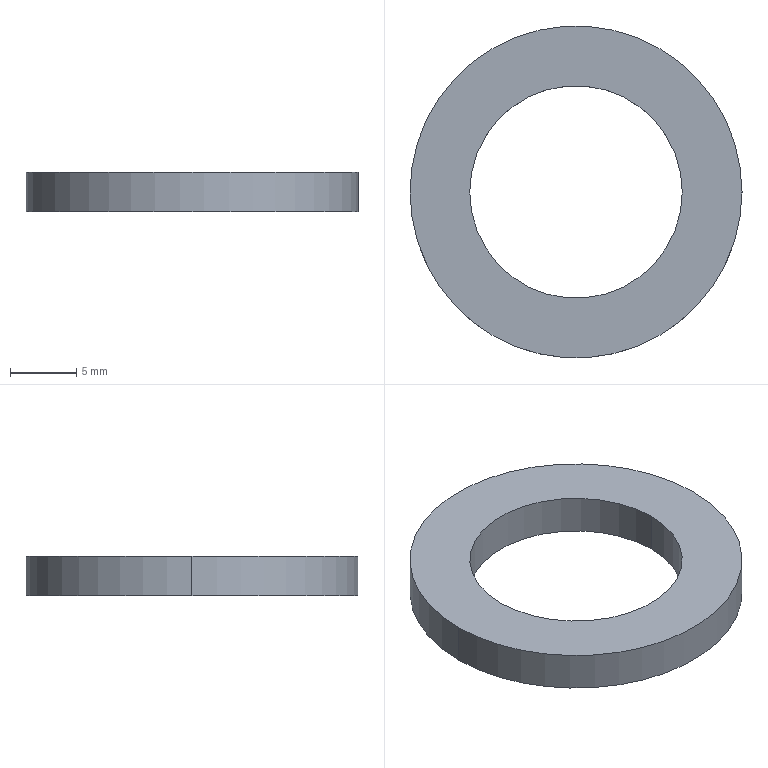Part | STEP file | Cuon T phu H01_17 | 1 solid | 6 faces | box 25 x 25 x 3 mm | volume 869.436 mm3 | cylinder 4 | plane 2 | commonest cylinder face diameters 16 x2 25 x2
STEP:
#1=CARTESIAN_POINT('',(0.,0.,0.));
#2=DIRECTION('',(0.,0.,1.));
#3=DIRECTION('',(1.,0.,0.));
#4=AXIS2_PLACEMENT_3D('',#1,#2,#3);
#5=CARTESIAN_POINT('',(-8.,0.,3.));
#6=VERTEX_POINT('',#5);
#7=CARTESIAN_POINT('',(-8.,0.,0.));
#8=VERTEX_POINT('',#7);
#9=CARTESIAN_POINT('',(-8.,0.,3.));
#10=DIRECTION('',(0.,0.,-1.));
#11=VECTOR('',#10,1.);
#12=LINE('',#9,#11);
#13=CARTESIAN_POINT('',(0.,0.,3.));
#14=DIRECTION('',(0.,0.,-1.));
#15=DIRECTION('',(-1.,0.,0.));
#16=AXIS2_PLACEMENT_3D('',#13,#14,#15);
#17=CYLINDRICAL_SURFACE('',#16,8.);
#18=CARTESIAN_POINT('',(6.283,0.));
#19=DIRECTION('',(0.,1.));
#20=VECTOR('',#19,1.);
#21=LINE('',#18,#20);
#22=(GEOMETRIC_REPRESENTATION_CONTEXT(2)PARAMETRIC_REPRESENTATION_CONTEXT()REPRESENTATION_CONTEXT('',''));
#23=DEFINITIONAL_REPRESENTATION('',(#21),#22);
#24=PCURVE('',#17,#23);
#25=CARTESIAN_POINT('',(0.,0.,3.));
#26=DIRECTION('',(0.,0.,-1.));
#27=DIRECTION('',(-1.,0.,0.));
#28=AXIS2_PLACEMENT_3D('',#25,#26,#27);
#29=CYLINDRICAL_SURFACE('',#28,8.);
#30=CARTESIAN_POINT('',(0.,0.));
#31=DIRECTION('',(0.,1.));
#32=VECTOR('',#31,1.);
#33=LINE('',#30,#32);
#34=(GEOMETRIC_REPRESENTATION_CONTEXT(2)PARAMETRIC_REPRESENTATION_CONTEXT()REPRESENTATION_CONTEXT('',''));
#35=DEFINITIONAL_REPRESENTATION('',(#33),#34);
#36=PCURVE('',#29,#35);
#37=SURFACE_CURVE('',#12,(#24,#36),.PCURVE_S1.);
#38=EDGE_CURVE('',#6,#8,#37,.T.);
#39=ORIENTED_EDGE('',*,*,#38,.T.);
#40=CARTESIAN_POINT('',(8.,0.,0.));
#41=VERTEX_POINT('',#40);
#42=CARTESIAN_POINT('',(0.,0.,0.));
#43=DIRECTION('',(0.,0.,1.));
#44=DIRECTION('',(1.,0.,0.));
#45=AXIS2_PLACEMENT_3D('',#42,#43,#44);
#46=CIRCLE('',#45,8.);
#47=CARTESIAN_POINT('',(9.425,3.));
#48=DIRECTION('',(-1.,0.));
#49=VECTOR('',#48,1.);
#50=LINE('',#47,#49);
#51=(GEOMETRIC_REPRESENTATION_CONTEXT(2)PARAMETRIC_REPRESENTATION_CONTEXT()REPRESENTATION_CONTEXT('',''));
#52=DEFINITIONAL_REPRESENTATION('',(#50),#51);
#53=PCURVE('',#17,#52);
#54=CARTESIAN_POINT('',(0.,0.,0.));
#55=DIRECTION('',(0.,0.,1.));
#56=DIRECTION('',(1.,0.,0.));
#57=AXIS2_PLACEMENT_3D('',#54,#55,#56);
#58=PLANE('',#57);
#59=CARTESIAN_POINT('',(0.,0.));
#60=DIRECTION('',(1.,0.));
#61=AXIS2_PLACEMENT_2D('',#59,#60);
#62=CIRCLE('',#61,8.);
#63=(GEOMETRIC_REPRESENTATION_CONTEXT(2)PARAMETRIC_REPRESENTATION_CONTEXT()REPRESENTATION_CONTEXT('',''));
#64=DEFINITIONAL_REPRESENTATION('',(#62),#63);
#65=PCURVE('',#58,#64);
#66=SURFACE_CURVE('',#46,(#53,#65),.PCURVE_S1.);
#67=EDGE_CURVE('',#8,#41,#66,.T.);
#68=ORIENTED_EDGE('',*,*,#67,.T.);
#69=CARTESIAN_POINT('',(8.,0.,3.));
#70=VERTEX_POINT('',#69);
#71=CARTESIAN_POINT('',(8.,0.,3.));
#72=DIRECTION('',(0.,0.,-1.));
#73=VECTOR('',#72,1.);
#74=LINE('',#71,#73);
#75=CARTESIAN_POINT('',(3.142,0.));
#76=DIRECTION('',(0.,1.));
#77=VECTOR('',#76,1.);
#78=LINE('',#75,#77);
#79=(GEOMETRIC_REPRESENTATION_CONTEXT(2)PARAMETRIC_REPRESENTATION_CONTEXT()REPRESENTATION_CONTEXT('',''));
#80=DEFINITIONAL_REPRESENTATION('',(#78),#79);
#81=PCURVE('',#17,#80);
#82=CARTESIAN_POINT('',(3.142,0.));
#83=DIRECTION('',(0.,1.));
#84=VECTOR('',#83,1.);
#85=LINE('',#82,#84);
#86=(GEOMETRIC_REPRESENTATION_CONTEXT(2)PARAMETRIC_REPRESENTATION_CONTEXT()REPRESENTATION_CONTEXT('',''));
#87=DEFINITIONAL_REPRESENTATION('',(#85),#86);
#88=PCURVE('',#29,#87);
#89=SURFACE_CURVE('',#74,(#81,#88),.PCURVE_S1.);
#90=EDGE_CURVE('',#70,#41,#89,.T.);
#91=ORIENTED_EDGE('',*,*,#90,.F.);
#92=CARTESIAN_POINT('',(0.,0.,3.));
#93=DIRECTION('',(0.,0.,1.));
#94=DIRECTION('',(1.,0.,0.));
#95=AXIS2_PLACEMENT_3D('',#92,#93,#94);
#96=CIRCLE('',#95,8.);
#97=CARTESIAN_POINT('',(9.425,0.));
#98=DIRECTION('',(-1.,0.));
#99=VECTOR('',#98,1.);
#100=LINE('',#97,#99);
#101=(GEOMETRIC_REPRESENTATION_CONTEXT(2)PARAMETRIC_REPRESENTATION_CONTEXT()REPRESENTATION_CONTEXT('',''));
#102=DEFINITIONAL_REPRESENTATION('',(#100),#101);
#103=PCURVE('',#17,#102);
#104=CARTESIAN_POINT('',(0.,0.,3.));
#105=DIRECTION('',(0.,0.,1.));
#106=DIRECTION('',(1.,0.,0.));
#107=AXIS2_PLACEMENT_3D('',#104,#105,#106);
#108=PLANE('',#107);
#109=CARTESIAN_POINT('',(0.,0.));
#110=DIRECTION('',(1.,0.));
#111=AXIS2_PLACEMENT_2D('',#109,#110);
#112=CIRCLE('',#111,8.);
#113=(GEOMETRIC_REPRESENTATION_CONTEXT(2)PARAMETRIC_REPRESENTATION_CONTEXT()REPRESENTATION_CONTEXT('',''));
#114=DEFINITIONAL_REPRESENTATION('',(#112),#113);
#115=PCURVE('',#108,#114);
#116=SURFACE_CURVE('',#96,(#103,#115),.PCURVE_S1.);
#117=EDGE_CURVE('',#6,#70,#116,.T.);
#118=ORIENTED_EDGE('',*,*,#117,.F.);
#119=EDGE_LOOP('',(#39,#68,#91,#118));
#120=FACE_BOUND('',#119,.F.);
#121=ADVANCED_FACE('',(#120),#17,.F.);
#122=CARTESIAN_POINT('',(12.5,0.,3.));
#123=VERTEX_POINT('',#122);
#124=CARTESIAN_POINT('',(-12.5,0.,3.));
#125=VERTEX_POINT('',#124);
#126=CARTESIAN_POINT('',(0.,0.,3.));
#127=DIRECTION('',(0.,0.,1.));
#128=DIRECTION('',(1.,0.,0.));
#129=AXIS2_PLACEMENT_3D('',#126,#127,#128);
#130=CIRCLE('',#129,12.5);
#131=CARTESIAN_POINT('',(0.,0.,3.));
#132=DIRECTION('',(0.,0.,-1.));
#133=DIRECTION('',(-1.,0.,0.));
#134=AXIS2_PLACEMENT_3D('',#131,#132,#133);
#135=CYLINDRICAL_SURFACE('',#134,12.5);
#136=CARTESIAN_POINT('',(3.142,0.));
#137=DIRECTION('',(-1.,0.));
#138=VECTOR('',#137,1.);
#139=LINE('',#136,#138);
#140=(GEOMETRIC_REPRESENTATION_CONTEXT(2)PARAMETRIC_REPRESENTATION_CONTEXT()REPRESENTATION_CONTEXT('',''));
#141=DEFINITIONAL_REPRESENTATION('',(#139),#140);
#142=PCURVE('',#135,#141);
#143=CARTESIAN_POINT('',(0.,0.));
#144=DIRECTION('',(1.,0.));
#145=AXIS2_PLACEMENT_2D('',#143,#144);
#146=CIRCLE('',#145,12.5);
#147=(GEOMETRIC_REPRESENTATION_CONTEXT(2)PARAMETRIC_REPRESENTATION_CONTEXT()REPRESENTATION_CONTEXT('',''));
#148=DEFINITIONAL_REPRESENTATION('',(#146),#147);
#149=PCURVE('',#108,#148);
#150=SURFACE_CURVE('',#130,(#142,#149),.PCURVE_S1.);
#151=EDGE_CURVE('',#123,#125,#150,.T.);
#152=ORIENTED_EDGE('',*,*,#151,.F.);
#153=CARTESIAN_POINT('',(12.5,0.,0.));
#154=VERTEX_POINT('',#153);
#155=CARTESIAN_POINT('',(12.5,0.,3.));
#156=DIRECTION('',(0.,0.,-1.));
#157=VECTOR('',#156,1.);
#158=LINE('',#155,#157);
#159=CARTESIAN_POINT('',(3.142,0.));
#160=DIRECTION('',(0.,1.));
#161=VECTOR('',#160,1.);
#162=LINE('',#159,#161);
#163=(GEOMETRIC_REPRESENTATION_CONTEXT(2)PARAMETRIC_REPRESENTATION_CONTEXT()REPRESENTATION_CONTEXT('',''));
#164=DEFINITIONAL_REPRESENTATION('',(#162),#163);
#165=PCURVE('',#135,#164);
#166=CARTESIAN_POINT('',(0.,0.,3.));
#167=DIRECTION('',(0.,0.,-1.));
#168=DIRECTION('',(-1.,0.,0.));
#169=AXIS2_PLACEMENT_3D('',#166,#167,#168);
#170=CYLINDRICAL_SURFACE('',#169,12.5);
#171=CARTESIAN_POINT('',(3.142,0.));
#172=DIRECTION('',(0.,1.));
#173=VECTOR('',#172,1.);
#174=LINE('',#171,#173);
#175=(GEOMETRIC_REPRESENTATION_CONTEXT(2)PARAMETRIC_REPRESENTATION_CONTEXT()REPRESENTATION_CONTEXT('',''));
#176=DEFINITIONAL_REPRESENTATION('',(#174),#175);
#177=PCURVE('',#170,#176);
#178=SURFACE_CURVE('',#158,(#165,#177),.PCURVE_S1.);
#179=EDGE_CURVE('',#123,#154,#178,.T.);
#180=ORIENTED_EDGE('',*,*,#179,.T.);
#181=CARTESIAN_POINT('',(-12.5,0.,0.));
#182=VERTEX_POINT('',#181);
#183=CARTESIAN_POINT('',(0.,0.,0.));
#184=DIRECTION('',(0.,0.,1.));
#185=DIRECTION('',(1.,0.,0.));
#186=AXIS2_PLACEMENT_3D('',#183,#184,#185);
#187=CIRCLE('',#186,12.5);
#188=CARTESIAN_POINT('',(3.142,3.));
#189=DIRECTION('',(-1.,0.));
#190=VECTOR('',#189,1.);
#191=LINE('',#188,#190);
#192=(GEOMETRIC_REPRESENTATION_CONTEXT(2)PARAMETRIC_REPRESENTATION_CONTEXT()REPRESENTATION_CONTEXT('',''));
#193=DEFINITIONAL_REPRESENTATION('',(#191),#192);
#194=PCURVE('',#135,#193);
#195=CARTESIAN_POINT('',(0.,0.));
#196=DIRECTION('',(1.,0.));
#197=AXIS2_PLACEMENT_2D('',#195,#196);
#198=CIRCLE('',#197,12.5);
#199=(GEOMETRIC_REPRESENTATION_CONTEXT(2)PARAMETRIC_REPRESENTATION_CONTEXT()REPRESENTATION_CONTEXT('',''));
#200=DEFINITIONAL_REPRESENTATION('',(#198),#199);
#201=PCURVE('',#58,#200);
#202=SURFACE_CURVE('',#187,(#194,#201),.PCURVE_S1.);
#203=EDGE_CURVE('',#154,#182,#202,.T.);
#204=ORIENTED_EDGE('',*,*,#203,.T.);
#205=CARTESIAN_POINT('',(-12.5,0.,3.));
#206=DIRECTION('',(0.,0.,-1.));
#207=VECTOR('',#206,1.);
#208=LINE('',#205,#207);
#209=CARTESIAN_POINT('',(0.,0.));
#210=DIRECTION('',(0.,1.));
#211=VECTOR('',#210,1.);
#212=LINE('',#209,#211);
#213=(GEOMETRIC_REPRESENTATION_CONTEXT(2)PARAMETRIC_REPRESENTATION_CONTEXT()REPRESENTATION_CONTEXT('',''));
#214=DEFINITIONAL_REPRESENTATION('',(#212),#213);
#215=PCURVE('',#135,#214);
#216=CARTESIAN_POINT('',(6.283,0.));
#217=DIRECTION('',(0.,1.));
#218=VECTOR('',#217,1.);
#219=LINE('',#216,#218);
#220=(GEOMETRIC_REPRESENTATION_CONTEXT(2)PARAMETRIC_REPRESENTATION_CONTEXT()REPRESENTATION_CONTEXT('',''));
#221=DEFINITIONAL_REPRESENTATION('',(#219),#220);
#222=PCURVE('',#170,#221);
#223=SURFACE_CURVE('',#208,(#215,#222),.PCURVE_S1.);
#224=EDGE_CURVE('',#125,#182,#223,.T.);
#225=ORIENTED_EDGE('',*,*,#224,.F.);
#226=EDGE_LOOP('',(#152,#180,#204,#225));
#227=FACE_BOUND('',#226,.T.);
#228=ADVANCED_FACE('',(#227),#135,.T.);
#229=CARTESIAN_POINT('',(0.,0.,3.));
#230=DIRECTION('',(0.,0.,1.));
#231=DIRECTION('',(1.,0.,0.));
#232=AXIS2_PLACEMENT_3D('',#229,#230,#231);
#233=CIRCLE('',#232,12.5);
#234=CARTESIAN_POINT('',(0.,0.));
#235=DIRECTION('',(1.,0.));
#236=AXIS2_PLACEMENT_2D('',#234,#235);
#237=CIRCLE('',#236,12.5);
#238=(GEOMETRIC_REPRESENTATION_CONTEXT(2)PARAMETRIC_REPRESENTATION_CONTEXT()REPRESENTATION_CONTEXT('',''));
#239=DEFINITIONAL_REPRESENTATION('',(#237),#238);
#240=PCURVE('',#108,#239);
#241=CARTESIAN_POINT('',(9.425,0.));
#242=DIRECTION('',(-1.,0.));
#243=VECTOR('',#242,1.);
#244=LINE('',#241,#243);
#245=(GEOMETRIC_REPRESENTATION_CONTEXT(2)PARAMETRIC_REPRESENTATION_CONTEXT()REPRESENTATION_CONTEXT('',''));
#246=DEFINITIONAL_REPRESENTATION('',(#244),#245);
#247=PCURVE('',#170,#246);
#248=SURFACE_CURVE('',#233,(#240,#247),.PCURVE_S1.);
#249=EDGE_CURVE('',#125,#123,#248,.T.);
#250=ORIENTED_EDGE('',*,*,#249,.T.);
#251=ORIENTED_EDGE('',*,*,#151,.T.);
#252=EDGE_LOOP('',(#250,#251));
#253=FACE_BOUND('',#252,.T.);
#254=ORIENTED_EDGE('',*,*,#117,.F.);
#255=CARTESIAN_POINT('',(0.,0.,3.));
#256=DIRECTION('',(0.,0.,1.));
#257=DIRECTION('',(1.,0.,0.));
#258=AXIS2_PLACEMENT_3D('',#255,#256,#257);
#259=CIRCLE('',#258,8.);
#260=CARTESIAN_POINT('',(0.,0.));
#261=DIRECTION('',(1.,0.));
#262=AXIS2_PLACEMENT_2D('',#260,#261);
#263=CIRCLE('',#262,8.);
#264=(GEOMETRIC_REPRESENTATION_CONTEXT(2)PARAMETRIC_REPRESENTATION_CONTEXT()REPRESENTATION_CONTEXT('',''));
#265=DEFINITIONAL_REPRESENTATION('',(#263),#264);
#266=PCURVE('',#108,#265);
#267=CARTESIAN_POINT('',(3.142,0.));
#268=DIRECTION('',(-1.,0.));
#269=VECTOR('',#268,1.);
#270=LINE('',#267,#269);
#271=(GEOMETRIC_REPRESENTATION_CONTEXT(2)PARAMETRIC_REPRESENTATION_CONTEXT()REPRESENTATION_CONTEXT('',''));
#272=DEFINITIONAL_REPRESENTATION('',(#270),#271);
#273=PCURVE('',#29,#272);
#274=SURFACE_CURVE('',#259,(#266,#273),.PCURVE_S1.);
#275=EDGE_CURVE('',#70,#6,#274,.T.);
#276=ORIENTED_EDGE('',*,*,#275,.F.);
#277=EDGE_LOOP('',(#254,#276));
#278=FACE_BOUND('',#277,.T.);
#279=ADVANCED_FACE('',(#253,#278),#108,.T.);
#280=CARTESIAN_POINT('',(0.,0.,0.));
#281=DIRECTION('',(0.,0.,1.));
#282=DIRECTION('',(1.,0.,0.));
#283=AXIS2_PLACEMENT_3D('',#280,#281,#282);
#284=CIRCLE('',#283,12.5);
#285=CARTESIAN_POINT('',(0.,0.));
#286=DIRECTION('',(1.,0.));
#287=AXIS2_PLACEMENT_2D('',#285,#286);
#288=CIRCLE('',#287,12.5);
#289=(GEOMETRIC_REPRESENTATION_CONTEXT(2)PARAMETRIC_REPRESENTATION_CONTEXT()REPRESENTATION_CONTEXT('',''));
#290=DEFINITIONAL_REPRESENTATION('',(#288),#289);
#291=PCURVE('',#58,#290);
#292=CARTESIAN_POINT('',(9.425,3.));
#293=DIRECTION('',(-1.,0.));
#294=VECTOR('',#293,1.);
#295=LINE('',#292,#294);
#296=(GEOMETRIC_REPRESENTATION_CONTEXT(2)PARAMETRIC_REPRESENTATION_CONTEXT()REPRESENTATION_CONTEXT('',''));
#297=DEFINITIONAL_REPRESENTATION('',(#295),#296);
#298=PCURVE('',#170,#297);
#299=SURFACE_CURVE('',#284,(#291,#298),.PCURVE_S1.);
#300=EDGE_CURVE('',#182,#154,#299,.T.);
#301=ORIENTED_EDGE('',*,*,#300,.F.);
#302=ORIENTED_EDGE('',*,*,#203,.F.);
#303=EDGE_LOOP('',(#301,#302));
#304=FACE_BOUND('',#303,.T.);
#305=ORIENTED_EDGE('',*,*,#67,.T.);
#306=CARTESIAN_POINT('',(0.,0.,0.));
#307=DIRECTION('',(0.,0.,1.));
#308=DIRECTION('',(1.,0.,0.));
#309=AXIS2_PLACEMENT_3D('',#306,#307,#308);
#310=CIRCLE('',#309,8.);
#311=CARTESIAN_POINT('',(0.,0.));
#312=DIRECTION('',(1.,0.));
#313=AXIS2_PLACEMENT_2D('',#311,#312);
#314=CIRCLE('',#313,8.);
#315=(GEOMETRIC_REPRESENTATION_CONTEXT(2)PARAMETRIC_REPRESENTATION_CONTEXT()REPRESENTATION_CONTEXT('',''));
#316=DEFINITIONAL_REPRESENTATION('',(#314),#315);
#317=PCURVE('',#58,#316);
#318=CARTESIAN_POINT('',(3.142,3.));
#319=DIRECTION('',(-1.,0.));
#320=VECTOR('',#319,1.);
#321=LINE('',#318,#320);
#322=(GEOMETRIC_REPRESENTATION_CONTEXT(2)PARAMETRIC_REPRESENTATION_CONTEXT()REPRESENTATION_CONTEXT('',''));
#323=DEFINITIONAL_REPRESENTATION('',(#321),#322);
#324=PCURVE('',#29,#323);
#325=SURFACE_CURVE('',#310,(#317,#324),.PCURVE_S1.);
#326=EDGE_CURVE('',#41,#8,#325,.T.);
#327=ORIENTED_EDGE('',*,*,#326,.T.);
#328=EDGE_LOOP('',(#305,#327));
#329=FACE_BOUND('',#328,.T.);
#330=ADVANCED_FACE('',(#304,#329),#58,.F.);
#331=ORIENTED_EDGE('',*,*,#179,.F.);
#332=ORIENTED_EDGE('',*,*,#249,.F.);
#333=ORIENTED_EDGE('',*,*,#224,.T.);
#334=ORIENTED_EDGE('',*,*,#300,.T.);
#335=EDGE_LOOP('',(#331,#332,#333,#334));
#336=FACE_BOUND('',#335,.T.);
#337=ADVANCED_FACE('',(#336),#170,.T.);
#338=ORIENTED_EDGE('',*,*,#326,.T.);
#339=ORIENTED_EDGE('',*,*,#38,.F.);
#340=ORIENTED_EDGE('',*,*,#275,.F.);
#341=ORIENTED_EDGE('',*,*,#90,.T.);
#342=EDGE_LOOP('',(#338,#339,#340,#341));
#343=FACE_BOUND('',#342,.F.);
#344=ADVANCED_FACE('',(#343),#29,.F.);
#345=CLOSED_SHELL('',(#121,#228,#279,#330,#337,#344));
#346=MANIFOLD_SOLID_BREP('',#345);
#347=(LENGTH_UNIT()NAMED_UNIT(*)SI_UNIT(.MILLI.,.METRE.));
#348=UNCERTAINTY_MEASURE_WITH_UNIT(LENGTH_MEASURE(0.0000001),#347,'','');
#349=(NAMED_UNIT(*)PLANE_ANGLE_UNIT()SI_UNIT($,.RADIAN.));
#350=(NAMED_UNIT(*)SI_UNIT($,.STERADIAN.)SOLID_ANGLE_UNIT());
#351=(GEOMETRIC_REPRESENTATION_CONTEXT(3)GLOBAL_UNCERTAINTY_ASSIGNED_CONTEXT((#348))GLOBAL_UNIT_ASSIGNED_CONTEXT((#347,#349,#350))REPRESENTATION_CONTEXT('',''));
#352=ADVANCED_BREP_SHAPE_REPRESENTATION('',(#4,#346),#351);